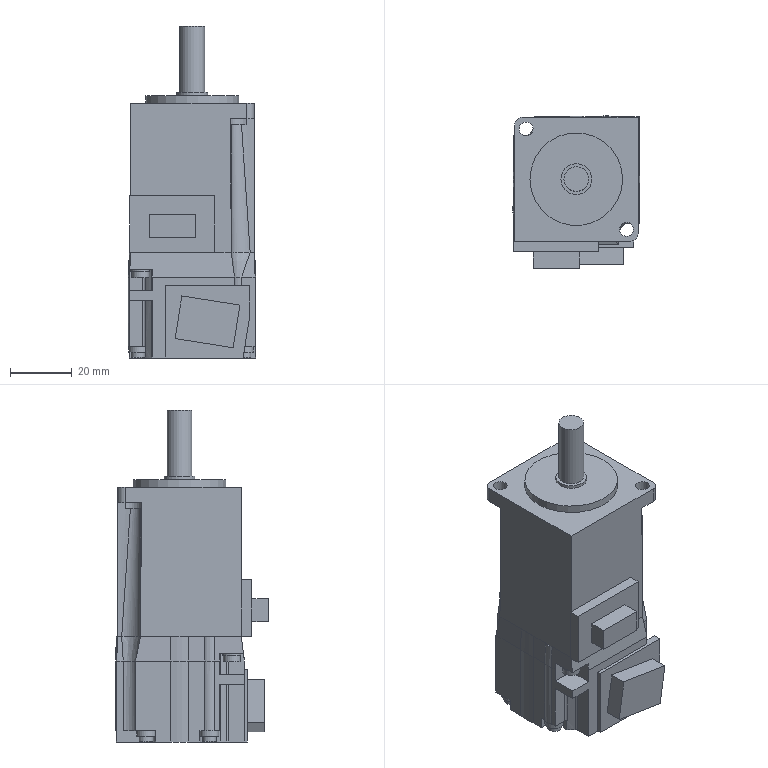Part | STEP file | hg-kr13_ | 1 solid | 163 faces | box 41.2 x 49.5 x 107.4 mm | volume 131615 mm3 | plane 106 | cylinder 46 | spline 9 | cone 2 | commonest cylinder face diameters 2 x8 4.5 x6 6 x4 6.2 x4 40.5 x4 8 x3